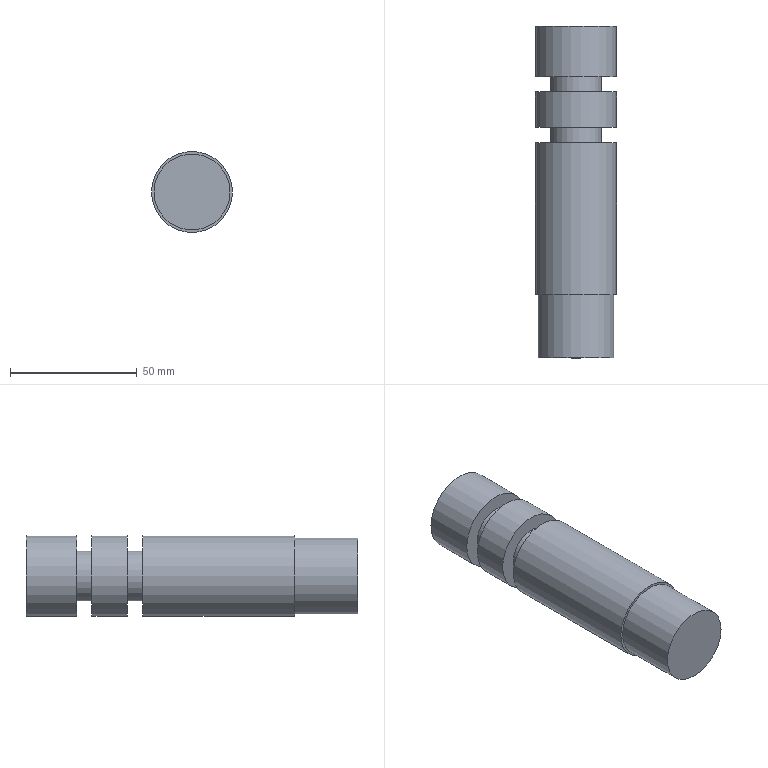Part | NX | features solid 2 | 1 solid | 13 faces | box 32 x 131 x 32 mm | volume 97041 mm3 | plane 7 | cylinder 6 | commonest cylinder face diameters 32 x3 20 x2 30 x1
STEP:
#1=CARTESIAN_POINT('',(-56.,530.,125.));
#2=VERTEX_POINT('',#1);
#3=CARTESIAN_POINT('',(-40.,530.,125.));
#4=DIRECTION('',(0.,1.,0.));
#5=DIRECTION('',(-1.,0.,0.));
#6=AXIS2_PLACEMENT_3D('',#3,#4,#5);
#7=CIRCLE('',#6,16.);
#8=EDGE_CURVE('',#2,#2,#7,.T.);
#9=ORIENTED_EDGE('',*,*,#8,.T.);
#10=EDGE_LOOP('',(#9));
#11=FACE_BOUND('',#10,.T.);
#12=CARTESIAN_POINT('',(-50.,530.,125.));
#13=VERTEX_POINT('',#12);
#14=CARTESIAN_POINT('',(-40.,530.,125.));
#15=DIRECTION('',(0.,1.,0.));
#16=DIRECTION('',(-1.,0.,0.));
#17=AXIS2_PLACEMENT_3D('',#14,#15,#16);
#18=CIRCLE('',#17,10.);
#19=EDGE_CURVE('',#13,#13,#18,.T.);
#20=ORIENTED_EDGE('',*,*,#19,.F.);
#21=EDGE_LOOP('',(#20));
#22=FACE_BOUND('',#21,.T.);
#23=CARTESIAN_POINT('',(-40.,530.,125.));
#24=DIRECTION('',(0.,1.,0.));
#25=DIRECTION('',(0.,0.,-1.));
#26=AXIS2_PLACEMENT_3D('',#23,#24,#25);
#27=PLANE('',#26);
#28=ADVANCED_FACE('',(#11,#22),#27,.T.);
#29=CARTESIAN_POINT('',(-56.,510.,125.));
#30=VERTEX_POINT('',#29);
#31=CARTESIAN_POINT('',(-40.,510.,125.));
#32=DIRECTION('',(0.,1.,0.));
#33=DIRECTION('',(-1.,0.,0.));
#34=AXIS2_PLACEMENT_3D('',#31,#32,#33);
#35=CIRCLE('',#34,16.);
#36=EDGE_CURVE('',#30,#30,#35,.T.);
#37=ORIENTED_EDGE('',*,*,#36,.T.);
#38=EDGE_LOOP('',(#37));
#39=FACE_BOUND('',#38,.T.);
#40=CARTESIAN_POINT('',(-50.,510.,125.));
#41=VERTEX_POINT('',#40);
#42=CARTESIAN_POINT('',(-40.,510.,125.));
#43=DIRECTION('',(0.,1.,0.));
#44=DIRECTION('',(-1.,0.,0.));
#45=AXIS2_PLACEMENT_3D('',#42,#43,#44);
#46=CIRCLE('',#45,10.);
#47=EDGE_CURVE('',#41,#41,#46,.T.);
#48=ORIENTED_EDGE('',*,*,#47,.F.);
#49=EDGE_LOOP('',(#48));
#50=FACE_BOUND('',#49,.T.);
#51=CARTESIAN_POINT('',(-40.,510.,125.));
#52=DIRECTION('',(0.,1.,0.));
#53=DIRECTION('',(0.,0.,-1.));
#54=AXIS2_PLACEMENT_3D('',#51,#52,#53);
#55=PLANE('',#54);
#56=ADVANCED_FACE('',(#39,#50),#55,.T.);
#57=ORIENTED_EDGE('',*,*,#36,.F.);
#58=EDGE_LOOP('',(#57));
#59=FACE_BOUND('',#58,.T.);
#60=CARTESIAN_POINT('',(-56.,450.,125.));
#61=VERTEX_POINT('',#60);
#62=CARTESIAN_POINT('',(-40.,450.,125.));
#63=DIRECTION('',(0.,1.,0.));
#64=DIRECTION('',(-1.,0.,0.));
#65=AXIS2_PLACEMENT_3D('',#62,#63,#64);
#66=CIRCLE('',#65,16.);
#67=EDGE_CURVE('',#61,#61,#66,.T.);
#68=ORIENTED_EDGE('',*,*,#67,.T.);
#69=EDGE_LOOP('',(#68));
#70=FACE_BOUND('',#69,.T.);
#71=CARTESIAN_POINT('',(-40.,510.,125.));
#72=DIRECTION('',(0.,-1.,0.));
#73=DIRECTION('',(0.,0.,1.));
#74=AXIS2_PLACEMENT_3D('',#71,#72,#73);
#75=CYLINDRICAL_SURFACE('',#74,16.);
#76=ADVANCED_FACE('',(#59,#70),#75,.T.);
#77=CARTESIAN_POINT('',(-55.,450.,125.));
#78=VERTEX_POINT('',#77);
#79=CARTESIAN_POINT('',(-40.,450.,125.));
#80=DIRECTION('',(0.,1.,0.));
#81=DIRECTION('',(-1.,0.,0.));
#82=AXIS2_PLACEMENT_3D('',#79,#80,#81);
#83=CIRCLE('',#82,15.);
#84=EDGE_CURVE('',#78,#78,#83,.T.);
#85=ORIENTED_EDGE('',*,*,#84,.T.);
#86=EDGE_LOOP('',(#85));
#87=FACE_BOUND('',#86,.T.);
#88=ORIENTED_EDGE('',*,*,#67,.F.);
#89=EDGE_LOOP('',(#88));
#90=FACE_BOUND('',#89,.T.);
#91=CARTESIAN_POINT('',(-40.,450.,125.));
#92=DIRECTION('',(0.,1.,0.));
#93=DIRECTION('',(0.,0.,-1.));
#94=AXIS2_PLACEMENT_3D('',#91,#92,#93);
#95=PLANE('',#94);
#96=ADVANCED_FACE('',(#87,#90),#95,.F.);
#97=CARTESIAN_POINT('',(-55.,425.,125.));
#98=VERTEX_POINT('',#97);
#99=CARTESIAN_POINT('',(-40.,425.,125.));
#100=DIRECTION('',(0.,1.,0.));
#101=DIRECTION('',(-1.,0.,0.));
#102=AXIS2_PLACEMENT_3D('',#99,#100,#101);
#103=CIRCLE('',#102,15.);
#104=EDGE_CURVE('',#98,#98,#103,.T.);
#105=ORIENTED_EDGE('',*,*,#104,.T.);
#106=EDGE_LOOP('',(#105));
#107=FACE_BOUND('',#106,.T.);
#108=ORIENTED_EDGE('',*,*,#84,.F.);
#109=EDGE_LOOP('',(#108));
#110=FACE_BOUND('',#109,.T.);
#111=CARTESIAN_POINT('',(-40.,425.,125.));
#112=DIRECTION('',(0.,1.,0.));
#113=DIRECTION('',(0.,0.,-1.));
#114=AXIS2_PLACEMENT_3D('',#111,#112,#113);
#115=CYLINDRICAL_SURFACE('',#114,15.);
#116=ADVANCED_FACE('',(#107,#110),#115,.T.);
#117=ORIENTED_EDGE('',*,*,#104,.F.);
#118=EDGE_LOOP('',(#117));
#119=FACE_BOUND('',#118,.T.);
#120=CARTESIAN_POINT('',(-40.,425.,125.));
#121=DIRECTION('',(0.,1.,0.));
#122=DIRECTION('',(0.,0.,-1.));
#123=AXIS2_PLACEMENT_3D('',#120,#121,#122);
#124=PLANE('',#123);
#125=ADVANCED_FACE('',(#119),#124,.F.);
#126=CARTESIAN_POINT('',(-50.,516.,125.));
#127=VERTEX_POINT('',#126);
#128=CARTESIAN_POINT('',(-40.,516.,125.));
#129=DIRECTION('',(0.,1.,0.));
#130=DIRECTION('',(-1.,0.,0.));
#131=AXIS2_PLACEMENT_3D('',#128,#129,#130);
#132=CIRCLE('',#131,10.);
#133=EDGE_CURVE('',#127,#127,#132,.T.);
#134=ORIENTED_EDGE('',*,*,#133,.F.);
#135=EDGE_LOOP('',(#134));
#136=FACE_BOUND('',#135,.T.);
#137=ORIENTED_EDGE('',*,*,#47,.T.);
#138=EDGE_LOOP('',(#137));
#139=FACE_BOUND('',#138,.T.);
#140=CARTESIAN_POINT('',(-40.,516.,125.));
#141=DIRECTION('',(0.,-1.,0.));
#142=DIRECTION('',(0.,0.,1.));
#143=AXIS2_PLACEMENT_3D('',#140,#141,#142);
#144=CYLINDRICAL_SURFACE('',#143,10.);
#145=ADVANCED_FACE('',(#136,#139),#144,.T.);
#146=CARTESIAN_POINT('',(-56.,516.,125.));
#147=VERTEX_POINT('',#146);
#148=CARTESIAN_POINT('',(-40.,516.,125.));
#149=DIRECTION('',(0.,1.,0.));
#150=DIRECTION('',(-1.,0.,0.));
#151=AXIS2_PLACEMENT_3D('',#148,#149,#150);
#152=CIRCLE('',#151,16.);
#153=EDGE_CURVE('',#147,#147,#152,.T.);
#154=ORIENTED_EDGE('',*,*,#153,.F.);
#155=EDGE_LOOP('',(#154));
#156=FACE_BOUND('',#155,.T.);
#157=ORIENTED_EDGE('',*,*,#133,.T.);
#158=EDGE_LOOP('',(#157));
#159=FACE_BOUND('',#158,.T.);
#160=CARTESIAN_POINT('',(-40.,516.,125.));
#161=DIRECTION('',(0.,1.,0.));
#162=DIRECTION('',(0.,0.,-1.));
#163=AXIS2_PLACEMENT_3D('',#160,#161,#162);
#164=PLANE('',#163);
#165=ADVANCED_FACE('',(#156,#159),#164,.F.);
#166=ORIENTED_EDGE('',*,*,#8,.F.);
#167=EDGE_LOOP('',(#166));
#168=FACE_BOUND('',#167,.T.);
#169=ORIENTED_EDGE('',*,*,#153,.T.);
#170=EDGE_LOOP('',(#169));
#171=FACE_BOUND('',#170,.T.);
#172=CARTESIAN_POINT('',(-40.,530.,125.));
#173=DIRECTION('',(0.,-1.,0.));
#174=DIRECTION('',(0.,0.,1.));
#175=AXIS2_PLACEMENT_3D('',#172,#173,#174);
#176=CYLINDRICAL_SURFACE('',#175,16.);
#177=ADVANCED_FACE('',(#168,#171),#176,.T.);
#178=CARTESIAN_POINT('',(-50.,536.,125.));
#179=VERTEX_POINT('',#178);
#180=CARTESIAN_POINT('',(-40.,536.,125.));
#181=DIRECTION('',(0.,1.,0.));
#182=DIRECTION('',(-1.,0.,0.));
#183=AXIS2_PLACEMENT_3D('',#180,#181,#182);
#184=CIRCLE('',#183,10.);
#185=EDGE_CURVE('',#179,#179,#184,.T.);
#186=ORIENTED_EDGE('',*,*,#185,.F.);
#187=EDGE_LOOP('',(#186));
#188=FACE_BOUND('',#187,.T.);
#189=ORIENTED_EDGE('',*,*,#19,.T.);
#190=EDGE_LOOP('',(#189));
#191=FACE_BOUND('',#190,.T.);
#192=CARTESIAN_POINT('',(-40.,536.,125.));
#193=DIRECTION('',(0.,-1.,0.));
#194=DIRECTION('',(0.,0.,1.));
#195=AXIS2_PLACEMENT_3D('',#192,#193,#194);
#196=CYLINDRICAL_SURFACE('',#195,10.);
#197=ADVANCED_FACE('',(#188,#191),#196,.T.);
#198=CARTESIAN_POINT('',(-56.,536.,125.));
#199=VERTEX_POINT('',#198);
#200=CARTESIAN_POINT('',(-40.,536.,125.));
#201=DIRECTION('',(0.,1.,0.));
#202=DIRECTION('',(-1.,0.,0.));
#203=AXIS2_PLACEMENT_3D('',#200,#201,#202);
#204=CIRCLE('',#203,16.);
#205=EDGE_CURVE('',#199,#199,#204,.T.);
#206=ORIENTED_EDGE('',*,*,#205,.F.);
#207=EDGE_LOOP('',(#206));
#208=FACE_BOUND('',#207,.T.);
#209=ORIENTED_EDGE('',*,*,#185,.T.);
#210=EDGE_LOOP('',(#209));
#211=FACE_BOUND('',#210,.T.);
#212=CARTESIAN_POINT('',(-40.,536.,125.));
#213=DIRECTION('',(0.,1.,0.));
#214=DIRECTION('',(0.,0.,-1.));
#215=AXIS2_PLACEMENT_3D('',#212,#213,#214);
#216=PLANE('',#215);
#217=ADVANCED_FACE('',(#208,#211),#216,.F.);
#218=CARTESIAN_POINT('',(-56.,556.,125.));
#219=VERTEX_POINT('',#218);
#220=CARTESIAN_POINT('',(-40.,556.,125.));
#221=DIRECTION('',(0.,1.,0.));
#222=DIRECTION('',(-1.,0.,0.));
#223=AXIS2_PLACEMENT_3D('',#220,#221,#222);
#224=CIRCLE('',#223,16.);
#225=EDGE_CURVE('',#219,#219,#224,.T.);
#226=ORIENTED_EDGE('',*,*,#225,.F.);
#227=EDGE_LOOP('',(#226));
#228=FACE_BOUND('',#227,.T.);
#229=ORIENTED_EDGE('',*,*,#205,.T.);
#230=EDGE_LOOP('',(#229));
#231=FACE_BOUND('',#230,.T.);
#232=CARTESIAN_POINT('',(-40.,556.,125.));
#233=DIRECTION('',(0.,-1.,0.));
#234=DIRECTION('',(0.,0.,1.));
#235=AXIS2_PLACEMENT_3D('',#232,#233,#234);
#236=CYLINDRICAL_SURFACE('',#235,16.);
#237=ADVANCED_FACE('',(#228,#231),#236,.T.);
#238=ORIENTED_EDGE('',*,*,#225,.T.);
#239=EDGE_LOOP('',(#238));
#240=FACE_BOUND('',#239,.T.);
#241=CARTESIAN_POINT('',(-40.,556.,125.));
#242=DIRECTION('',(0.,1.,0.));
#243=DIRECTION('',(0.,0.,-1.));
#244=AXIS2_PLACEMENT_3D('',#241,#242,#243);
#245=PLANE('',#244);
#246=ADVANCED_FACE('',(#240),#245,.T.);
#247=CLOSED_SHELL('',(#28,#56,#76,#96,#116,#125,#145,#165,#177,#197,#217,#237,#246));
#248=MANIFOLD_SOLID_BREP('',#247);
#249=(LENGTH_UNIT()NAMED_UNIT(*)SI_UNIT(.MILLI.,.METRE.));
#250=UNCERTAINTY_MEASURE_WITH_UNIT(LENGTH_MEASURE(0.00001),#249,'','');
#251=(NAMED_UNIT(*)PLANE_ANGLE_UNIT()SI_UNIT($,.RADIAN.));
#252=(NAMED_UNIT(*)SI_UNIT($,.STERADIAN.)SOLID_ANGLE_UNIT());
#253=(GEOMETRIC_REPRESENTATION_CONTEXT(3)GLOBAL_UNCERTAINTY_ASSIGNED_CONTEXT((#250))GLOBAL_UNIT_ASSIGNED_CONTEXT((#249,#251,#252))REPRESENTATION_CONTEXT('',''));
#254=ADVANCED_BREP_SHAPE_REPRESENTATION('',(#248),#253);